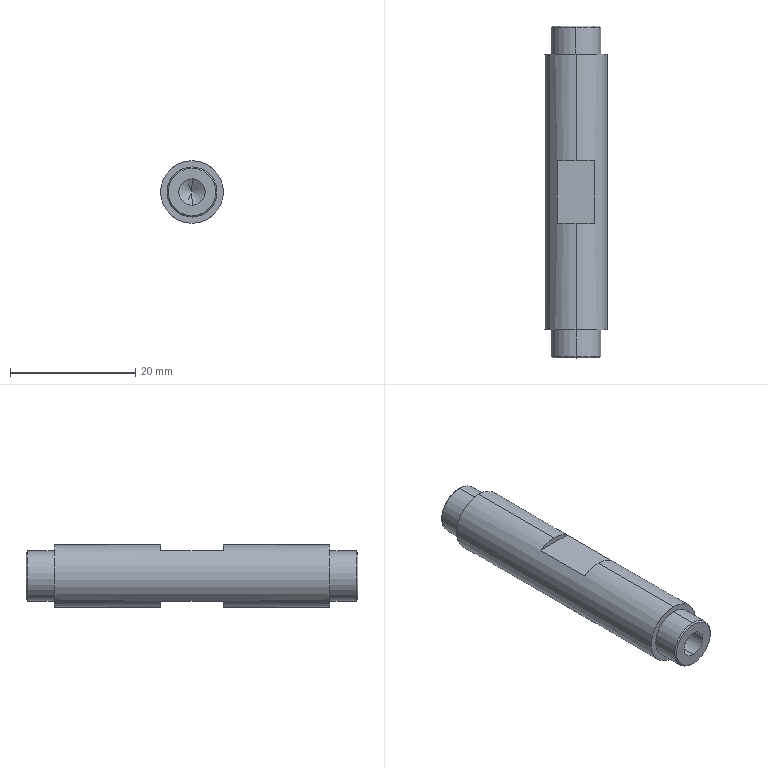Part | SolidWorks | features ICE 3, Chamfer 1, HoleWzd 1, MirrorPattern 1, Revolution 1 | 1 solid | 28 faces | box 10 x 53 x 10 mm | volume 3526 mm3 | cylinder 10 | plane 10 | cone 8 | commonest cylinder face diameters 4.2 x4 8 x4 10 x2
STEP:
#1=CARTESIAN_POINT('',(0.,26.5,3.8));
#2=VERTEX_POINT('',#1);
#3=CARTESIAN_POINT('',(0.,26.5,-3.8));
#4=VERTEX_POINT('',#3);
#5=CARTESIAN_POINT('',(0.,26.5,0.));
#6=DIRECTION('',(0.,1.,0.));
#7=DIRECTION('',(0.,0.,1.));
#8=AXIS2_PLACEMENT_3D('',#5,#6,#7);
#9=CIRCLE('',#8,3.8);
#10=EDGE_CURVE('',#2,#4,#9,.T.);
#11=ORIENTED_EDGE('',*,*,#10,.F.);
#12=CARTESIAN_POINT('',(0.,26.3,4.));
#13=VERTEX_POINT('',#12);
#14=CARTESIAN_POINT('',(0.,26.5,3.8));
#15=DIRECTION('',(0.,-0.7071,0.7071));
#16=VECTOR('',#15,1000.);
#17=LINE('',#14,#16);
#18=EDGE_CURVE('',#2,#13,#17,.T.);
#19=ORIENTED_EDGE('',*,*,#18,.T.);
#20=CARTESIAN_POINT('',(0.,26.3,-4.));
#21=VERTEX_POINT('',#20);
#22=CARTESIAN_POINT('',(0.,26.3,0.));
#23=DIRECTION('',(0.,-1.,0.));
#24=DIRECTION('',(0.,0.,1.));
#25=AXIS2_PLACEMENT_3D('',#22,#23,#24);
#26=CIRCLE('',#25,4.);
#27=EDGE_CURVE('',#21,#13,#26,.T.);
#28=ORIENTED_EDGE('',*,*,#27,.F.);
#29=CARTESIAN_POINT('',(0.,26.5,-3.8));
#30=DIRECTION('',(0.,-0.7071,-0.7071));
#31=VECTOR('',#30,1000.);
#32=LINE('',#29,#31);
#33=EDGE_CURVE('',#4,#21,#32,.T.);
#34=ORIENTED_EDGE('',*,*,#33,.F.);
#35=EDGE_LOOP('',(#11,#19,#28,#34));
#36=FACE_OUTER_BOUND('',#35,.T.);
#37=CARTESIAN_POINT('',(0.,26.5,0.));
#38=DIRECTION('',(0.,-1.,0.));
#39=DIRECTION('',(0.,0.,-1.));
#40=AXIS2_PLACEMENT_3D('',#37,#38,#39);
#41=CONICAL_SURFACE('',#40,3.8,0.7854);
#42=ADVANCED_FACE('',(#36),#41,.T.);
#43=CARTESIAN_POINT('',(0.,-26.5,-3.8));
#44=VERTEX_POINT('',#43);
#45=CARTESIAN_POINT('',(0.,-26.5,3.8));
#46=VERTEX_POINT('',#45);
#47=CARTESIAN_POINT('',(0.,-26.5,0.));
#48=DIRECTION('',(0.,-1.,0.));
#49=DIRECTION('',(0.,0.,-1.));
#50=AXIS2_PLACEMENT_3D('',#47,#48,#49);
#51=CIRCLE('',#50,3.8);
#52=EDGE_CURVE('',#44,#46,#51,.T.);
#53=ORIENTED_EDGE('',*,*,#52,.F.);
#54=CARTESIAN_POINT('',(0.,-26.3,-4.));
#55=VERTEX_POINT('',#54);
#56=CARTESIAN_POINT('',(0.,-26.5,-3.8));
#57=DIRECTION('',(0.,0.7071,-0.7071));
#58=VECTOR('',#57,1000.);
#59=LINE('',#56,#58);
#60=EDGE_CURVE('',#44,#55,#59,.T.);
#61=ORIENTED_EDGE('',*,*,#60,.T.);
#62=CARTESIAN_POINT('',(0.,-26.3,4.));
#63=VERTEX_POINT('',#62);
#64=CARTESIAN_POINT('',(0.,-26.3,0.));
#65=DIRECTION('',(0.,1.,0.));
#66=DIRECTION('',(0.,0.,-1.));
#67=AXIS2_PLACEMENT_3D('',#64,#65,#66);
#68=CIRCLE('',#67,4.);
#69=EDGE_CURVE('',#63,#55,#68,.T.);
#70=ORIENTED_EDGE('',*,*,#69,.F.);
#71=CARTESIAN_POINT('',(0.,-26.5,3.8));
#72=DIRECTION('',(0.,0.7071,0.7071));
#73=VECTOR('',#72,1000.);
#74=LINE('',#71,#73);
#75=EDGE_CURVE('',#46,#63,#74,.T.);
#76=ORIENTED_EDGE('',*,*,#75,.F.);
#77=EDGE_LOOP('',(#53,#61,#70,#76));
#78=FACE_OUTER_BOUND('',#77,.T.);
#79=CARTESIAN_POINT('',(0.,-26.5,0.));
#80=DIRECTION('',(0.,1.,0.));
#81=DIRECTION('',(0.,0.,1.));
#82=AXIS2_PLACEMENT_3D('',#79,#80,#81);
#83=CONICAL_SURFACE('',#82,3.8,0.7854);
#84=ADVANCED_FACE('',(#78),#83,.T.);
#85=CARTESIAN_POINT('',(0.,16.1,-2.1));
#86=VERTEX_POINT('',#85);
#87=CARTESIAN_POINT('',(0.,16.1,2.1));
#88=VERTEX_POINT('',#87);
#89=CARTESIAN_POINT('',(0.,16.1,0.));
#90=DIRECTION('',(0.,1.,0.));
#91=DIRECTION('',(0.,0.,1.));
#92=AXIS2_PLACEMENT_3D('',#89,#90,#91);
#93=CIRCLE('',#92,2.1);
#94=EDGE_CURVE('',#86,#88,#93,.T.);
#95=ORIENTED_EDGE('',*,*,#94,.F.);
#96=CARTESIAN_POINT('',(0.,26.5,-2.1));
#97=VERTEX_POINT('',#96);
#98=CARTESIAN_POINT('',(0.,26.5,-2.1));
#99=DIRECTION('',(0.,1.,0.));
#100=VECTOR('',#99,1000.);
#101=LINE('',#98,#100);
#102=EDGE_CURVE('',#86,#97,#101,.T.);
#103=ORIENTED_EDGE('',*,*,#102,.T.);
#104=CARTESIAN_POINT('',(0.,26.5,2.1));
#105=VERTEX_POINT('',#104);
#106=CARTESIAN_POINT('',(0.,26.5,0.));
#107=DIRECTION('',(0.,1.,0.));
#108=DIRECTION('',(0.,0.,1.));
#109=AXIS2_PLACEMENT_3D('',#106,#107,#108);
#110=CIRCLE('',#109,2.1);
#111=EDGE_CURVE('',#97,#105,#110,.T.);
#112=ORIENTED_EDGE('',*,*,#111,.T.);
#113=CARTESIAN_POINT('',(0.,26.5,2.1));
#114=DIRECTION('',(0.,1.,0.));
#115=VECTOR('',#114,1000.);
#116=LINE('',#113,#115);
#117=EDGE_CURVE('',#88,#105,#116,.T.);
#118=ORIENTED_EDGE('',*,*,#117,.F.);
#119=EDGE_LOOP('',(#95,#103,#112,#118));
#120=FACE_OUTER_BOUND('',#119,.T.);
#121=CARTESIAN_POINT('',(0.,26.5,0.));
#122=DIRECTION('',(0.,1.,0.));
#123=DIRECTION('',(0.,0.,1.));
#124=AXIS2_PLACEMENT_3D('',#121,#122,#123);
#125=CYLINDRICAL_SURFACE('',#124,2.1);
#126=ADVANCED_FACE('',(#120),#125,.F.);
#127=CARTESIAN_POINT('',(0.,14.838,0.));
#128=VERTEX_POINT('',#127);
#129=CARTESIAN_POINT('',(0.,16.1,2.1));
#130=DIRECTION('',(0.,0.515,0.8572));
#131=VECTOR('',#130,1000.);
#132=LINE('',#129,#131);
#133=EDGE_CURVE('',#128,#88,#132,.T.);
#134=ORIENTED_EDGE('',*,*,#133,.F.);
#135=CARTESIAN_POINT('',(0.,16.1,-2.1));
#136=DIRECTION('',(0.,0.515,-0.8572));
#137=VECTOR('',#136,1000.);
#138=LINE('',#135,#137);
#139=EDGE_CURVE('',#128,#86,#138,.T.);
#140=ORIENTED_EDGE('',*,*,#139,.T.);
#141=ORIENTED_EDGE('',*,*,#94,.T.);
#142=EDGE_LOOP('',(#134,#140,#141));
#143=FACE_OUTER_BOUND('',#142,.T.);
#144=CARTESIAN_POINT('',(0.,16.1,0.));
#145=DIRECTION('',(0.,1.,0.));
#146=DIRECTION('',(0.,0.,1.));
#147=AXIS2_PLACEMENT_3D('',#144,#145,#146);
#148=CONICAL_SURFACE('',#147,2.1,1.03);
#149=ADVANCED_FACE('',(#143),#148,.F.);
#150=CARTESIAN_POINT('',(0.,22.,4.));
#151=VERTEX_POINT('',#150);
#152=CARTESIAN_POINT('',(0.,22.,-4.));
#153=VERTEX_POINT('',#152);
#154=CARTESIAN_POINT('',(0.,22.,0.));
#155=DIRECTION('',(0.,1.,0.));
#156=DIRECTION('',(0.,0.,1.));
#157=AXIS2_PLACEMENT_3D('',#154,#155,#156);
#158=CIRCLE('',#157,4.);
#159=EDGE_CURVE('',#151,#153,#158,.T.);
#160=ORIENTED_EDGE('',*,*,#159,.T.);
#161=CARTESIAN_POINT('',(0.,22.,-4.));
#162=DIRECTION('',(0.,1.,0.));
#163=VECTOR('',#162,1000.);
#164=LINE('',#161,#163);
#165=EDGE_CURVE('',#153,#21,#164,.T.);
#166=ORIENTED_EDGE('',*,*,#165,.T.);
#167=ORIENTED_EDGE('',*,*,#27,.T.);
#168=CARTESIAN_POINT('',(0.,22.,4.));
#169=DIRECTION('',(0.,1.,0.));
#170=VECTOR('',#169,1000.);
#171=LINE('',#168,#170);
#172=EDGE_CURVE('',#151,#13,#171,.T.);
#173=ORIENTED_EDGE('',*,*,#172,.F.);
#174=EDGE_LOOP('',(#160,#166,#167,#173));
#175=FACE_OUTER_BOUND('',#174,.T.);
#176=CARTESIAN_POINT('',(0.,22.,0.));
#177=DIRECTION('',(0.,1.,0.));
#178=DIRECTION('',(0.,0.,1.));
#179=AXIS2_PLACEMENT_3D('',#176,#177,#178);
#180=CYLINDRICAL_SURFACE('',#179,4.);
#181=ADVANCED_FACE('',(#175),#180,.T.);
#182=CARTESIAN_POINT('',(0.,-16.1,2.1));
#183=VERTEX_POINT('',#182);
#184=CARTESIAN_POINT('',(0.,-16.1,-2.1));
#185=VERTEX_POINT('',#184);
#186=CARTESIAN_POINT('',(0.,-16.1,0.));
#187=DIRECTION('',(0.,-1.,0.));
#188=DIRECTION('',(0.,0.,-1.));
#189=AXIS2_PLACEMENT_3D('',#186,#187,#188);
#190=CIRCLE('',#189,2.1);
#191=EDGE_CURVE('',#183,#185,#190,.T.);
#192=ORIENTED_EDGE('',*,*,#191,.F.);
#193=CARTESIAN_POINT('',(0.,-26.5,2.1));
#194=VERTEX_POINT('',#193);
#195=CARTESIAN_POINT('',(0.,-26.5,2.1));
#196=DIRECTION('',(0.,-1.,0.));
#197=VECTOR('',#196,1000.);
#198=LINE('',#195,#197);
#199=EDGE_CURVE('',#183,#194,#198,.T.);
#200=ORIENTED_EDGE('',*,*,#199,.T.);
#201=CARTESIAN_POINT('',(0.,-26.5,-2.1));
#202=VERTEX_POINT('',#201);
#203=CARTESIAN_POINT('',(0.,-26.5,0.));
#204=DIRECTION('',(0.,-1.,0.));
#205=DIRECTION('',(0.,0.,-1.));
#206=AXIS2_PLACEMENT_3D('',#203,#204,#205);
#207=CIRCLE('',#206,2.1);
#208=EDGE_CURVE('',#194,#202,#207,.T.);
#209=ORIENTED_EDGE('',*,*,#208,.T.);
#210=CARTESIAN_POINT('',(0.,-26.5,-2.1));
#211=DIRECTION('',(0.,-1.,0.));
#212=VECTOR('',#211,1000.);
#213=LINE('',#210,#212);
#214=EDGE_CURVE('',#185,#202,#213,.T.);
#215=ORIENTED_EDGE('',*,*,#214,.F.);
#216=EDGE_LOOP('',(#192,#200,#209,#215));
#217=FACE_OUTER_BOUND('',#216,.T.);
#218=CARTESIAN_POINT('',(0.,-26.5,0.));
#219=DIRECTION('',(0.,-1.,0.));
#220=DIRECTION('',(0.,0.,-1.));
#221=AXIS2_PLACEMENT_3D('',#218,#219,#220);
#222=CYLINDRICAL_SURFACE('',#221,2.1);
#223=ADVANCED_FACE('',(#217),#222,.F.);
#224=CARTESIAN_POINT('',(0.,-14.838,0.));
#225=VERTEX_POINT('',#224);
#226=CARTESIAN_POINT('',(0.,-16.1,-2.1));
#227=DIRECTION('',(0.,-0.515,-0.8572));
#228=VECTOR('',#227,1000.);
#229=LINE('',#226,#228);
#230=EDGE_CURVE('',#225,#185,#229,.T.);
#231=ORIENTED_EDGE('',*,*,#230,.F.);
#232=CARTESIAN_POINT('',(0.,-16.1,2.1));
#233=DIRECTION('',(0.,-0.515,0.8572));
#234=VECTOR('',#233,1000.);
#235=LINE('',#232,#234);
#236=EDGE_CURVE('',#225,#183,#235,.T.);
#237=ORIENTED_EDGE('',*,*,#236,.T.);
#238=ORIENTED_EDGE('',*,*,#191,.T.);
#239=EDGE_LOOP('',(#231,#237,#238));
#240=FACE_OUTER_BOUND('',#239,.T.);
#241=CARTESIAN_POINT('',(0.,-16.1,0.));
#242=DIRECTION('',(0.,-1.,0.));
#243=DIRECTION('',(0.,0.,-1.));
#244=AXIS2_PLACEMENT_3D('',#241,#242,#243);
#245=CONICAL_SURFACE('',#244,2.1,1.03);
#246=ADVANCED_FACE('',(#240),#245,.F.);
#247=CARTESIAN_POINT('',(0.,-22.,-4.));
#248=VERTEX_POINT('',#247);
#249=CARTESIAN_POINT('',(0.,-22.,4.));
#250=VERTEX_POINT('',#249);
#251=CARTESIAN_POINT('',(0.,-22.,0.));
#252=DIRECTION('',(0.,-1.,0.));
#253=DIRECTION('',(0.,0.,-1.));
#254=AXIS2_PLACEMENT_3D('',#251,#252,#253);
#255=CIRCLE('',#254,4.);
#256=EDGE_CURVE('',#248,#250,#255,.T.);
#257=ORIENTED_EDGE('',*,*,#256,.T.);
#258=CARTESIAN_POINT('',(0.,-22.,4.));
#259=DIRECTION('',(0.,-1.,0.));
#260=VECTOR('',#259,1000.);
#261=LINE('',#258,#260);
#262=EDGE_CURVE('',#250,#63,#261,.T.);
#263=ORIENTED_EDGE('',*,*,#262,.T.);
#264=ORIENTED_EDGE('',*,*,#69,.T.);
#265=CARTESIAN_POINT('',(0.,-22.,-4.));
#266=DIRECTION('',(0.,-1.,0.));
#267=VECTOR('',#266,1000.);
#268=LINE('',#265,#267);
#269=EDGE_CURVE('',#248,#55,#268,.T.);
#270=ORIENTED_EDGE('',*,*,#269,.F.);
#271=EDGE_LOOP('',(#257,#263,#264,#270));
#272=FACE_OUTER_BOUND('',#271,.T.);
#273=CARTESIAN_POINT('',(0.,-22.,0.));
#274=DIRECTION('',(0.,-1.,0.));
#275=DIRECTION('',(0.,0.,-1.));
#276=AXIS2_PLACEMENT_3D('',#273,#274,#275);
#277=CYLINDRICAL_SURFACE('',#276,4.);
#278=ADVANCED_FACE('',(#272),#277,.T.);
#279=CARTESIAN_POINT('',(0.,-22.,5.));
#280=VERTEX_POINT('',#279);
#281=CARTESIAN_POINT('',(0.,-22.,-5.));
#282=VERTEX_POINT('',#281);
#283=CARTESIAN_POINT('',(0.,-22.,0.));
#284=DIRECTION('',(0.,1.,0.));
#285=DIRECTION('',(0.,0.,-1.));
#286=AXIS2_PLACEMENT_3D('',#283,#284,#285);
#287=CIRCLE('',#286,5.);
#288=EDGE_CURVE('',#280,#282,#287,.T.);
#289=ORIENTED_EDGE('',*,*,#288,.T.);
#290=CARTESIAN_POINT('',(0.,-5.,-5.));
#291=VERTEX_POINT('',#290);
#292=CARTESIAN_POINT('',(0.,26.5,-5.));
#293=DIRECTION('',(0.,1.,0.));
#294=VECTOR('',#293,1000.);
#295=LINE('',#292,#294);
#296=EDGE_CURVE('',#282,#291,#295,.T.);
#297=ORIENTED_EDGE('',*,*,#296,.T.);
#298=CARTESIAN_POINT('',(3.,-5.,-4.));
#299=VERTEX_POINT('',#298);
#300=CARTESIAN_POINT('',(0.,-5.,0.));
#301=DIRECTION('',(0.,1.,0.));
#302=DIRECTION('',(0.,0.,-1.));
#303=AXIS2_PLACEMENT_3D('',#300,#301,#302);
#304=CIRCLE('',#303,5.);
#305=EDGE_CURVE('',#299,#291,#304,.T.);
#306=ORIENTED_EDGE('',*,*,#305,.F.);
#307=CARTESIAN_POINT('',(3.,5.,-4.));
#308=VERTEX_POINT('',#307);
#309=CARTESIAN_POINT('',(3.,26.5,-4.));
#310=DIRECTION('',(0.,-1.,0.));
#311=VECTOR('',#310,1000.);
#312=LINE('',#309,#311);
#313=EDGE_CURVE('',#308,#299,#312,.T.);
#314=ORIENTED_EDGE('',*,*,#313,.F.);
#315=CARTESIAN_POINT('',(0.,5.,-5.));
#316=VERTEX_POINT('',#315);
#317=CARTESIAN_POINT('',(0.,5.,0.));
#318=DIRECTION('',(0.,-1.,0.));
#319=DIRECTION('',(0.,0.,1.));
#320=AXIS2_PLACEMENT_3D('',#317,#318,#319);
#321=CIRCLE('',#320,5.);
#322=EDGE_CURVE('',#316,#308,#321,.T.);
#323=ORIENTED_EDGE('',*,*,#322,.F.);
#324=CARTESIAN_POINT('',(0.,22.,-5.));
#325=VERTEX_POINT('',#324);
#326=CARTESIAN_POINT('',(0.,26.5,-5.));
#327=DIRECTION('',(0.,1.,0.));
#328=VECTOR('',#327,1000.);
#329=LINE('',#326,#328);
#330=EDGE_CURVE('',#316,#325,#329,.T.);
#331=ORIENTED_EDGE('',*,*,#330,.T.);
#332=CARTESIAN_POINT('',(0.,22.,5.));
#333=VERTEX_POINT('',#332);
#334=CARTESIAN_POINT('',(0.,22.,0.));
#335=DIRECTION('',(0.,-1.,0.));
#336=DIRECTION('',(0.,0.,1.));
#337=AXIS2_PLACEMENT_3D('',#334,#335,#336);
#338=CIRCLE('',#337,5.);
#339=EDGE_CURVE('',#325,#333,#338,.T.);
#340=ORIENTED_EDGE('',*,*,#339,.T.);
#341=CARTESIAN_POINT('',(0.,5.,5.));
#342=VERTEX_POINT('',#341);
#343=CARTESIAN_POINT('',(0.,26.5,5.));
#344=DIRECTION('',(0.,1.,0.));
#345=VECTOR('',#344,1000.);
#346=LINE('',#343,#345);
#347=EDGE_CURVE('',#342,#333,#346,.T.);
#348=ORIENTED_EDGE('',*,*,#347,.F.);
#349=CARTESIAN_POINT('',(3.,5.,4.));
#350=VERTEX_POINT('',#349);
#351=CARTESIAN_POINT('',(0.,5.,0.));
#352=DIRECTION('',(0.,-1.,0.));
#353=DIRECTION('',(0.,0.,1.));
#354=AXIS2_PLACEMENT_3D('',#351,#352,#353);
#355=CIRCLE('',#354,5.);
#356=EDGE_CURVE('',#350,#342,#355,.T.);
#357=ORIENTED_EDGE('',*,*,#356,.F.);
#358=CARTESIAN_POINT('',(3.,-5.,4.));
#359=VERTEX_POINT('',#358);
#360=CARTESIAN_POINT('',(3.,26.5,4.));
#361=DIRECTION('',(0.,1.,0.));
#362=VECTOR('',#361,1000.);
#363=LINE('',#360,#362);
#364=EDGE_CURVE('',#359,#350,#363,.T.);
#365=ORIENTED_EDGE('',*,*,#364,.F.);
#366=CARTESIAN_POINT('',(0.,-5.,5.));
#367=VERTEX_POINT('',#366);
#368=CARTESIAN_POINT('',(0.,-5.,0.));
#369=DIRECTION('',(0.,1.,0.));
#370=DIRECTION('',(0.,0.,-1.));
#371=AXIS2_PLACEMENT_3D('',#368,#369,#370);
#372=CIRCLE('',#371,5.);
#373=EDGE_CURVE('',#367,#359,#372,.T.);
#374=ORIENTED_EDGE('',*,*,#373,.F.);
#375=CARTESIAN_POINT('',(0.,26.5,5.));
#376=DIRECTION('',(0.,1.,0.));
#377=VECTOR('',#376,1000.);
#378=LINE('',#375,#377);
#379=EDGE_CURVE('',#280,#367,#378,.T.);
#380=ORIENTED_EDGE('',*,*,#379,.F.);
#381=EDGE_LOOP('',(#289,#297,#306,#314,#323,#331,#340,#348,#357,#365,#374,#380));
#382=FACE_OUTER_BOUND('',#381,.T.);
#383=CARTESIAN_POINT('',(0.,26.5,0.));
#384=DIRECTION('',(0.,1.,0.));
#385=DIRECTION('',(0.,0.,1.));
#386=AXIS2_PLACEMENT_3D('',#383,#384,#385);
#387=CYLINDRICAL_SURFACE('',#386,5.);
#388=ADVANCED_FACE('',(#382),#387,.T.);
#389=ORIENTED_EDGE('',*,*,#296,.F.);
#390=CARTESIAN_POINT('',(0.,-22.,0.));
#391=DIRECTION('',(0.,1.,0.));
#392=DIRECTION('',(0.,0.,-1.));
#393=AXIS2_PLACEMENT_3D('',#390,#391,#392);
#394=CIRCLE('',#393,5.);
#395=EDGE_CURVE('',#282,#280,#394,.T.);
#396=ORIENTED_EDGE('',*,*,#395,.T.);
#397=ORIENTED_EDGE('',*,*,#379,.T.);
#398=CARTESIAN_POINT('',(-3.,-5.,4.));
#399=VERTEX_POINT('',#398);
#400=CARTESIAN_POINT('',(0.,-5.,0.));
#401=DIRECTION('',(0.,1.,0.));
#402=DIRECTION('',(0.,0.,-1.));
#403=AXIS2_PLACEMENT_3D('',#400,#401,#402);
#404=CIRCLE('',#403,5.);
#405=EDGE_CURVE('',#399,#367,#404,.T.);
#406=ORIENTED_EDGE('',*,*,#405,.F.);
#407=CARTESIAN_POINT('',(-3.,5.,4.));
#408=VERTEX_POINT('',#407);
#409=CARTESIAN_POINT('',(-3.,26.5,4.));
#410=DIRECTION('',(0.,-1.,0.));
#411=VECTOR('',#410,1000.);
#412=LINE('',#409,#411);
#413=EDGE_CURVE('',#408,#399,#412,.T.);
#414=ORIENTED_EDGE('',*,*,#413,.F.);
#415=CARTESIAN_POINT('',(0.,5.,0.));
#416=DIRECTION('',(0.,-1.,0.));
#417=DIRECTION('',(0.,0.,1.));
#418=AXIS2_PLACEMENT_3D('',#415,#416,#417);
#419=CIRCLE('',#418,5.);
#420=EDGE_CURVE('',#342,#408,#419,.T.);
#421=ORIENTED_EDGE('',*,*,#420,.F.);
#422=ORIENTED_EDGE('',*,*,#347,.T.);
#423=CARTESIAN_POINT('',(0.,22.,0.));
#424=DIRECTION('',(0.,-1.,0.));
#425=DIRECTION('',(0.,0.,1.));
#426=AXIS2_PLACEMENT_3D('',#423,#424,#425);
#427=CIRCLE('',#426,5.);
#428=EDGE_CURVE('',#333,#325,#427,.T.);
#429=ORIENTED_EDGE('',*,*,#428,.T.);
#430=ORIENTED_EDGE('',*,*,#330,.F.);
#431=CARTESIAN_POINT('',(-3.,5.,-4.));
#432=VERTEX_POINT('',#431);
#433=CARTESIAN_POINT('',(0.,5.,0.));
#434=DIRECTION('',(0.,-1.,0.));
#435=DIRECTION('',(0.,0.,1.));
#436=AXIS2_PLACEMENT_3D('',#433,#434,#435);
#437=CIRCLE('',#436,5.);
#438=EDGE_CURVE('',#432,#316,#437,.T.);
#439=ORIENTED_EDGE('',*,*,#438,.F.);
#440=CARTESIAN_POINT('',(-3.,-5.,-4.));
#441=VERTEX_POINT('',#440);
#442=CARTESIAN_POINT('',(-3.,26.5,-4.));
#443=DIRECTION('',(0.,1.,0.));
#444=VECTOR('',#443,1000.);
#445=LINE('',#442,#444);
#446=EDGE_CURVE('',#441,#432,#445,.T.);
#447=ORIENTED_EDGE('',*,*,#446,.F.);
#448=CARTESIAN_POINT('',(0.,-5.,0.));
#449=DIRECTION('',(0.,1.,0.));
#450=DIRECTION('',(0.,0.,-1.));
#451=AXIS2_PLACEMENT_3D('',#448,#449,#450);
#452=CIRCLE('',#451,5.);
#453=EDGE_CURVE('',#291,#441,#452,.T.);
#454=ORIENTED_EDGE('',*,*,#453,.F.);
#455=EDGE_LOOP('',(#389,#396,#397,#406,#414,#421,#422,#429,#430,#439,#447,#454));
#456=FACE_OUTER_BOUND('',#455,.T.);
#457=CARTESIAN_POINT('',(0.,26.5,0.));
#458=DIRECTION('',(0.,1.,0.));
#459=DIRECTION('',(0.,0.,1.));
#460=AXIS2_PLACEMENT_3D('',#457,#458,#459);
#461=CYLINDRICAL_SURFACE('',#460,5.);
#462=ADVANCED_FACE('',(#456),#461,.T.);
#463=ORIENTED_EDGE('',*,*,#288,.F.);
#464=ORIENTED_EDGE('',*,*,#395,.F.);
#465=EDGE_LOOP('',(#463,#464));
#466=FACE_OUTER_BOUND('',#465,.T.);
#467=ORIENTED_EDGE('',*,*,#256,.F.);
#468=CARTESIAN_POINT('',(0.,-22.,0.));
#469=DIRECTION('',(0.,-1.,0.));
#470=DIRECTION('',(0.,0.,-1.));
#471=AXIS2_PLACEMENT_3D('',#468,#469,#470);
#472=CIRCLE('',#471,4.);
#473=EDGE_CURVE('',#250,#248,#472,.T.);
#474=ORIENTED_EDGE('',*,*,#473,.F.);
#475=EDGE_LOOP('',(#467,#474));
#476=FACE_BOUND('',#475,.T.);
#477=CARTESIAN_POINT('',(0.,-22.,0.));
#478=DIRECTION('',(0.,-1.,0.));
#479=DIRECTION('',(0.,0.,-1.));
#480=AXIS2_PLACEMENT_3D('',#477,#478,#479);
#481=PLANE('',#480);
#482=ADVANCED_FACE('',(#466,#476),#481,.T.);
#483=ORIENTED_EDGE('',*,*,#262,.F.);
#484=ORIENTED_EDGE('',*,*,#473,.T.);
#485=ORIENTED_EDGE('',*,*,#269,.T.);
#486=CARTESIAN_POINT('',(0.,-26.3,0.));
#487=DIRECTION('',(0.,1.,0.));
#488=DIRECTION('',(0.,0.,-1.));
#489=AXIS2_PLACEMENT_3D('',#486,#487,#488);
#490=CIRCLE('',#489,4.);
#491=EDGE_CURVE('',#55,#63,#490,.T.);
#492=ORIENTED_EDGE('',*,*,#491,.T.);
#493=EDGE_LOOP('',(#483,#484,#485,#492));
#494=FACE_OUTER_BOUND('',#493,.T.);
#495=CARTESIAN_POINT('',(0.,-22.,0.));
#496=DIRECTION('',(0.,-1.,0.));
#497=DIRECTION('',(0.,0.,-1.));
#498=AXIS2_PLACEMENT_3D('',#495,#496,#497);
#499=CYLINDRICAL_SURFACE('',#498,4.);
#500=ADVANCED_FACE('',(#494),#499,.T.);
#501=ORIENTED_EDGE('',*,*,#236,.F.);
#502=ORIENTED_EDGE('',*,*,#230,.T.);
#503=CARTESIAN_POINT('',(0.,-16.1,0.));
#504=DIRECTION('',(0.,-1.,0.));
#505=DIRECTION('',(0.,0.,-1.));
#506=AXIS2_PLACEMENT_3D('',#503,#504,#505);
#507=CIRCLE('',#506,2.1);
#508=EDGE_CURVE('',#185,#183,#507,.T.);
#509=ORIENTED_EDGE('',*,*,#508,.T.);
#510=EDGE_LOOP('',(#501,#502,#509));
#511=FACE_OUTER_BOUND('',#510,.T.);
#512=CARTESIAN_POINT('',(0.,-16.1,0.));
#513=DIRECTION('',(0.,-1.,0.));
#514=DIRECTION('',(0.,0.,-1.));
#515=AXIS2_PLACEMENT_3D('',#512,#513,#514);
#516=CONICAL_SURFACE('',#515,2.1,1.03);
#517=ADVANCED_FACE('',(#511),#516,.F.);
#518=ORIENTED_EDGE('',*,*,#199,.F.);
#519=ORIENTED_EDGE('',*,*,#508,.F.);
#520=ORIENTED_EDGE('',*,*,#214,.T.);
#521=CARTESIAN_POINT('',(0.,-26.5,0.));
#522=DIRECTION('',(0.,-1.,0.));
#523=DIRECTION('',(0.,0.,-1.));
#524=AXIS2_PLACEMENT_3D('',#521,#522,#523);
#525=CIRCLE('',#524,2.1);
#526=EDGE_CURVE('',#202,#194,#525,.T.);
#527=ORIENTED_EDGE('',*,*,#526,.T.);
#528=EDGE_LOOP('',(#518,#519,#520,#527));
#529=FACE_OUTER_BOUND('',#528,.T.);
#530=CARTESIAN_POINT('',(0.,-26.5,0.));
#531=DIRECTION('',(0.,-1.,0.));
#532=DIRECTION('',(0.,0.,-1.));
#533=AXIS2_PLACEMENT_3D('',#530,#531,#532);
#534=CYLINDRICAL_SURFACE('',#533,2.1);
#535=ADVANCED_FACE('',(#529),#534,.F.);
#536=CARTESIAN_POINT('',(0.,-26.5,0.));
#537=DIRECTION('',(0.,-1.,0.));
#538=DIRECTION('',(0.,0.,-1.));
#539=AXIS2_PLACEMENT_3D('',#536,#537,#538);
#540=CIRCLE('',#539,3.8);
#541=EDGE_CURVE('',#46,#44,#540,.T.);
#542=ORIENTED_EDGE('',*,*,#541,.T.);
#543=ORIENTED_EDGE('',*,*,#52,.T.);
#544=EDGE_LOOP('',(#542,#543));
#545=FACE_OUTER_BOUND('',#544,.T.);
#546=ORIENTED_EDGE('',*,*,#526,.F.);
#547=ORIENTED_EDGE('',*,*,#208,.F.);
#548=EDGE_LOOP('',(#546,#547));
#549=FACE_BOUND('',#548,.T.);
#550=CARTESIAN_POINT('',(0.,-26.5,5.));
#551=DIRECTION('',(0.,-1.,0.));
#552=DIRECTION('',(0.,0.,-1.));
#553=AXIS2_PLACEMENT_3D('',#550,#551,#552);
#554=PLANE('',#553);
#555=ADVANCED_FACE('',(#545,#549),#554,.T.);
#556=ORIENTED_EDGE('',*,*,#428,.F.);
#557=ORIENTED_EDGE('',*,*,#339,.F.);
#558=EDGE_LOOP('',(#556,#557));
#559=FACE_OUTER_BOUND('',#558,.T.);
#560=ORIENTED_EDGE('',*,*,#159,.F.);
#561=CARTESIAN_POINT('',(0.,22.,0.));
#562=DIRECTION('',(0.,1.,0.));
#563=DIRECTION('',(0.,0.,1.));
#564=AXIS2_PLACEMENT_3D('',#561,#562,#563);
#565=CIRCLE('',#564,4.);
#566=EDGE_CURVE('',#153,#151,#565,.T.);
#567=ORIENTED_EDGE('',*,*,#566,.F.);
#568=EDGE_LOOP('',(#560,#567));
#569=FACE_BOUND('',#568,.T.);
#570=CARTESIAN_POINT('',(0.,22.,0.));
#571=DIRECTION('',(0.,1.,0.));
#572=DIRECTION('',(0.,0.,1.));
#573=AXIS2_PLACEMENT_3D('',#570,#571,#572);
#574=PLANE('',#573);
#575=ADVANCED_FACE('',(#559,#569),#574,.T.);
#576=ORIENTED_EDGE('',*,*,#165,.F.);
#577=ORIENTED_EDGE('',*,*,#566,.T.);
#578=ORIENTED_EDGE('',*,*,#172,.T.);
#579=CARTESIAN_POINT('',(0.,26.3,0.));
#580=DIRECTION('',(0.,-1.,0.));
#581=DIRECTION('',(0.,0.,1.));
#582=AXIS2_PLACEMENT_3D('',#579,#580,#581);
#583=CIRCLE('',#582,4.);
#584=EDGE_CURVE('',#13,#21,#583,.T.);
#585=ORIENTED_EDGE('',*,*,#584,.T.);
#586=EDGE_LOOP('',(#576,#577,#578,#585));
#587=FACE_OUTER_BOUND('',#586,.T.);
#588=CARTESIAN_POINT('',(0.,22.,0.));
#589=DIRECTION('',(0.,1.,0.));
#590=DIRECTION('',(0.,0.,1.));
#591=AXIS2_PLACEMENT_3D('',#588,#589,#590);
#592=CYLINDRICAL_SURFACE('',#591,4.);
#593=ADVANCED_FACE('',(#587),#592,.T.);
#594=ORIENTED_EDGE('',*,*,#139,.F.);
#595=ORIENTED_EDGE('',*,*,#133,.T.);
#596=CARTESIAN_POINT('',(0.,16.1,0.));
#597=DIRECTION('',(0.,1.,0.));
#598=DIRECTION('',(0.,0.,1.));
#599=AXIS2_PLACEMENT_3D('',#596,#597,#598);
#600=CIRCLE('',#599,2.1);
#601=EDGE_CURVE('',#88,#86,#600,.T.);
#602=ORIENTED_EDGE('',*,*,#601,.T.);
#603=EDGE_LOOP('',(#594,#595,#602));
#604=FACE_OUTER_BOUND('',#603,.T.);
#605=CARTESIAN_POINT('',(0.,16.1,0.));
#606=DIRECTION('',(0.,1.,0.));
#607=DIRECTION('',(0.,0.,1.));
#608=AXIS2_PLACEMENT_3D('',#605,#606,#607);
#609=CONICAL_SURFACE('',#608,2.1,1.03);
#610=ADVANCED_FACE('',(#604),#609,.F.);
#611=ORIENTED_EDGE('',*,*,#102,.F.);
#612=ORIENTED_EDGE('',*,*,#601,.F.);
#613=ORIENTED_EDGE('',*,*,#117,.T.);
#614=CARTESIAN_POINT('',(0.,26.5,0.));
#615=DIRECTION('',(0.,1.,0.));
#616=DIRECTION('',(0.,0.,1.));
#617=AXIS2_PLACEMENT_3D('',#614,#615,#616);
#618=CIRCLE('',#617,2.1);
#619=EDGE_CURVE('',#105,#97,#618,.T.);
#620=ORIENTED_EDGE('',*,*,#619,.T.);
#621=EDGE_LOOP('',(#611,#612,#613,#620));
#622=FACE_OUTER_BOUND('',#621,.T.);
#623=CARTESIAN_POINT('',(0.,26.5,0.));
#624=DIRECTION('',(0.,1.,0.));
#625=DIRECTION('',(0.,0.,1.));
#626=AXIS2_PLACEMENT_3D('',#623,#624,#625);
#627=CYLINDRICAL_SURFACE('',#626,2.1);
#628=ADVANCED_FACE('',(#622),#627,.F.);
#629=CARTESIAN_POINT('',(0.,26.5,0.));
#630=DIRECTION('',(0.,1.,0.));
#631=DIRECTION('',(0.,0.,1.));
#632=AXIS2_PLACEMENT_3D('',#629,#630,#631);
#633=CIRCLE('',#632,3.8);
#634=EDGE_CURVE('',#4,#2,#633,.T.);
#635=ORIENTED_EDGE('',*,*,#634,.T.);
#636=ORIENTED_EDGE('',*,*,#10,.T.);
#637=EDGE_LOOP('',(#635,#636));
#638=FACE_OUTER_BOUND('',#637,.T.);
#639=ORIENTED_EDGE('',*,*,#619,.F.);
#640=ORIENTED_EDGE('',*,*,#111,.F.);
#641=EDGE_LOOP('',(#639,#640));
#642=FACE_BOUND('',#641,.T.);
#643=CARTESIAN_POINT('',(0.,26.5,5.));
#644=DIRECTION('',(0.,1.,0.));
#645=DIRECTION('',(0.,0.,1.));
#646=AXIS2_PLACEMENT_3D('',#643,#644,#645);
#647=PLANE('',#646);
#648=ADVANCED_FACE('',(#638,#642),#647,.T.);
#649=ORIENTED_EDGE('',*,*,#356,.T.);
#650=ORIENTED_EDGE('',*,*,#420,.T.);
#651=CARTESIAN_POINT('',(-5.,5.,4.));
#652=DIRECTION('',(1.,0.,0.));
#653=VECTOR('',#652,1000.);
#654=LINE('',#651,#653);
#655=EDGE_CURVE('',#408,#350,#654,.T.);
#656=ORIENTED_EDGE('',*,*,#655,.T.);
#657=EDGE_LOOP('',(#649,#650,#656));
#658=FACE_OUTER_BOUND('',#657,.T.);
#659=CARTESIAN_POINT('',(-5.,5.,11.231));
#660=DIRECTION('',(0.,1.,0.));
#661=DIRECTION('',(0.,0.,1.));
#662=AXIS2_PLACEMENT_3D('',#659,#660,#661);
#663=PLANE('',#662);
#664=ADVANCED_FACE('',(#658),#663,.F.);
#665=ORIENTED_EDGE('',*,*,#413,.T.);
#666=CARTESIAN_POINT('',(-5.,-5.,4.));
#667=DIRECTION('',(1.,0.,0.));
#668=VECTOR('',#667,1000.);
#669=LINE('',#666,#668);
#670=EDGE_CURVE('',#399,#359,#669,.T.);
#671=ORIENTED_EDGE('',*,*,#670,.T.);
#672=ORIENTED_EDGE('',*,*,#364,.T.);
#673=ORIENTED_EDGE('',*,*,#655,.F.);
#674=EDGE_LOOP('',(#665,#671,#672,#673));
#675=FACE_OUTER_BOUND('',#674,.T.);
#676=CARTESIAN_POINT('',(-5.,5.,4.));
#677=DIRECTION('',(0.,0.,-1.));
#678=DIRECTION('',(-1.,0.,0.));
#679=AXIS2_PLACEMENT_3D('',#676,#677,#678);
#680=PLANE('',#679);
#681=ADVANCED_FACE('',(#675),#680,.F.);
#682=ORIENTED_EDGE('',*,*,#405,.T.);
#683=ORIENTED_EDGE('',*,*,#373,.T.);
#684=ORIENTED_EDGE('',*,*,#670,.F.);
#685=EDGE_LOOP('',(#682,#683,#684));
#686=FACE_OUTER_BOUND('',#685,.T.);
#687=CARTESIAN_POINT('',(-5.,-5.,11.231));
#688=DIRECTION('',(0.,-1.,0.));
#689=DIRECTION('',(0.,0.,-1.));
#690=AXIS2_PLACEMENT_3D('',#687,#688,#689);
#691=PLANE('',#690);
#692=ADVANCED_FACE('',(#686),#691,.F.);
#693=ORIENTED_EDGE('',*,*,#305,.T.);
#694=ORIENTED_EDGE('',*,*,#453,.T.);
#695=CARTESIAN_POINT('',(-5.,-5.,-4.));
#696=DIRECTION('',(1.,0.,0.));
#697=VECTOR('',#696,1000.);
#698=LINE('',#695,#697);
#699=EDGE_CURVE('',#441,#299,#698,.T.);
#700=ORIENTED_EDGE('',*,*,#699,.T.);
#701=EDGE_LOOP('',(#693,#694,#700));
#702=FACE_OUTER_BOUND('',#701,.T.);
#703=CARTESIAN_POINT('',(-5.,-5.,-6.607));
#704=DIRECTION('',(0.,-1.,0.));
#705=DIRECTION('',(0.,0.,-1.));
#706=AXIS2_PLACEMENT_3D('',#703,#704,#705);
#707=PLANE('',#706);
#708=ADVANCED_FACE('',(#702),#707,.F.);
#709=ORIENTED_EDGE('',*,*,#313,.T.);
#710=ORIENTED_EDGE('',*,*,#699,.F.);
#711=ORIENTED_EDGE('',*,*,#446,.T.);
#712=CARTESIAN_POINT('',(-5.,5.,-4.));
#713=DIRECTION('',(1.,0.,0.));
#714=VECTOR('',#713,1000.);
#715=LINE('',#712,#714);
#716=EDGE_CURVE('',#432,#308,#715,.T.);
#717=ORIENTED_EDGE('',*,*,#716,.T.);
#718=EDGE_LOOP('',(#709,#710,#711,#717));
#719=FACE_OUTER_BOUND('',#718,.T.);
#720=CARTESIAN_POINT('',(-5.,5.,-4.));
#721=DIRECTION('',(0.,0.,1.));
#722=DIRECTION('',(1.,0.,0.));
#723=AXIS2_PLACEMENT_3D('',#720,#721,#722);
#724=PLANE('',#723);
#725=ADVANCED_FACE('',(#719),#724,.F.);
#726=ORIENTED_EDGE('',*,*,#438,.T.);
#727=ORIENTED_EDGE('',*,*,#322,.T.);
#728=ORIENTED_EDGE('',*,*,#716,.F.);
#729=EDGE_LOOP('',(#726,#727,#728));
#730=FACE_OUTER_BOUND('',#729,.T.);
#731=CARTESIAN_POINT('',(-5.,5.,-6.607));
#732=DIRECTION('',(0.,1.,0.));
#733=DIRECTION('',(0.,0.,1.));
#734=AXIS2_PLACEMENT_3D('',#731,#732,#733);
#735=PLANE('',#734);
#736=ADVANCED_FACE('',(#730),#735,.F.);
#737=ORIENTED_EDGE('',*,*,#60,.F.);
#738=ORIENTED_EDGE('',*,*,#541,.F.);
#739=ORIENTED_EDGE('',*,*,#75,.T.);
#740=ORIENTED_EDGE('',*,*,#491,.F.);
#741=EDGE_LOOP('',(#737,#738,#739,#740));
#742=FACE_OUTER_BOUND('',#741,.T.);
#743=CARTESIAN_POINT('',(0.,-26.5,0.));
#744=DIRECTION('',(0.,1.,0.));
#745=DIRECTION('',(0.,0.,1.));
#746=AXIS2_PLACEMENT_3D('',#743,#744,#745);
#747=CONICAL_SURFACE('',#746,3.8,0.7854);
#748=ADVANCED_FACE('',(#742),#747,.T.);
#749=ORIENTED_EDGE('',*,*,#18,.F.);
#750=ORIENTED_EDGE('',*,*,#634,.F.);
#751=ORIENTED_EDGE('',*,*,#33,.T.);
#752=ORIENTED_EDGE('',*,*,#584,.F.);
#753=EDGE_LOOP('',(#749,#750,#751,#752));
#754=FACE_OUTER_BOUND('',#753,.T.);
#755=CARTESIAN_POINT('',(0.,26.5,0.));
#756=DIRECTION('',(0.,-1.,0.));
#757=DIRECTION('',(0.,0.,-1.));
#758=AXIS2_PLACEMENT_3D('',#755,#756,#757);
#759=CONICAL_SURFACE('',#758,3.8,0.7854);
#760=ADVANCED_FACE('',(#754),#759,.T.);
#761=CLOSED_SHELL('',(#42,#84,#126,#149,#181,#223,#246,#278,#388,#462,#482,#500,#517,#535,#555,#575,#593,#610,#628,#648,#664,#681,#692,#708,#725,#736,#748,#760));
#762=MANIFOLD_SOLID_BREP('',#761);
#763=CARTESIAN_POINT('',(0.,0.,0.));
#764=DIRECTION('',(0.,0.,1.));
#765=DIRECTION('',(1.,0.,0.));
#766=AXIS2_PLACEMENT_3D('',#763,#764,#765);
#767=(LENGTH_UNIT()NAMED_UNIT(*)SI_UNIT(.MILLI.,.METRE.));
#768=UNCERTAINTY_MEASURE_WITH_UNIT(LENGTH_MEASURE(0.00001),#767,'','');
#769=(NAMED_UNIT(*)PLANE_ANGLE_UNIT()SI_UNIT($,.RADIAN.));
#770=(NAMED_UNIT(*)SI_UNIT($,.STERADIAN.)SOLID_ANGLE_UNIT());
#771=(GEOMETRIC_REPRESENTATION_CONTEXT(3)GLOBAL_UNCERTAINTY_ASSIGNED_CONTEXT((#768))GLOBAL_UNIT_ASSIGNED_CONTEXT((#767,#769,#770))REPRESENTATION_CONTEXT('',''));
#772=ADVANCED_BREP_SHAPE_REPRESENTATION('',(#762,#766),#771);